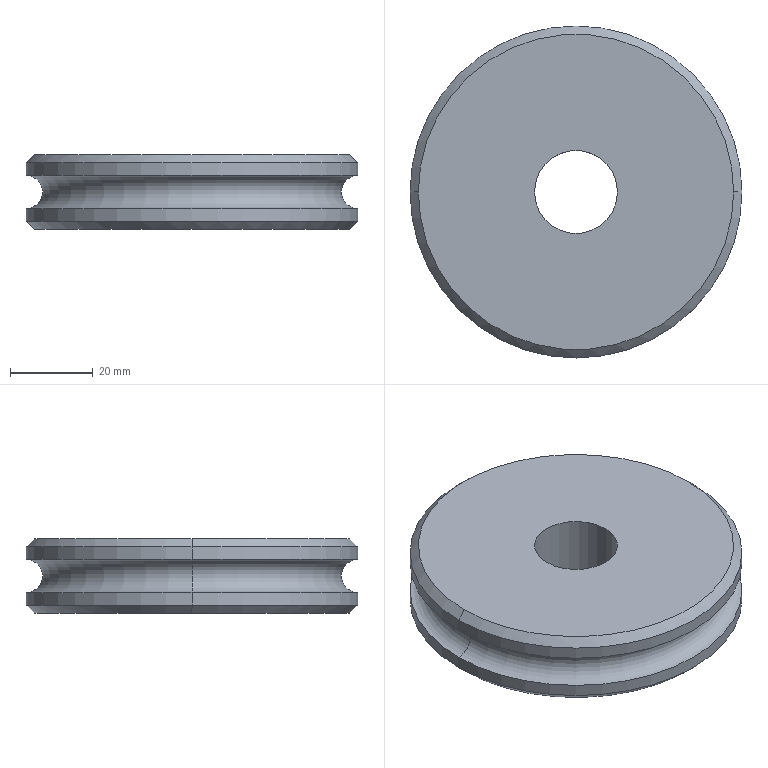Part | Creo | features DATUM PLANE 3, CHAMFER 1, COORDINATE SYSTEM 1, CURVE 1, CUT 1, PROTRUSION 1 | 1 solid | 14 faces | box 80 x 80 x 18 mm | volume 77786 mm3 | cylinder 6 | cone 4 | plane 2 | torus 2 | commonest cylinder face diameters 80 x4 20 x2
STEP:
#1=CARTESIAN_POINT('',(0.,0.,0.));
#2=DIRECTION('',(0.,0.,1.));
#3=DIRECTION('',(1.,0.,0.));
#4=AXIS2_PLACEMENT_3D('',#1,#2,#3);
#5=CARTESIAN_POINT('',(38.,0.,0.));
#6=VERTEX_POINT('',#5);
#7=CARTESIAN_POINT('',(-38.,0.,0.));
#8=VERTEX_POINT('',#7);
#9=CARTESIAN_POINT('',(0.,0.,0.));
#10=DIRECTION('',(0.,0.,-1.));
#11=DIRECTION('',(1.,0.,0.));
#12=AXIS2_PLACEMENT_3D('',#9,#10,#11);
#13=CIRCLE('',#12,38.);
#14=EDGE_CURVE('',#6,#8,#13,.T.);
#15=ORIENTED_EDGE('',*,*,#14,.F.);
#16=CARTESIAN_POINT('',(0.,0.,0.));
#17=DIRECTION('',(0.,0.,-1.));
#18=DIRECTION('',(-1.,0.,0.));
#19=AXIS2_PLACEMENT_3D('',#16,#17,#18);
#20=CIRCLE('',#19,38.);
#21=EDGE_CURVE('',#8,#6,#20,.T.);
#22=ORIENTED_EDGE('',*,*,#21,.F.);
#23=EDGE_LOOP('',(#15,#22));
#24=FACE_OUTER_BOUND('',#23,.F.);
#25=CARTESIAN_POINT('',(10.,0.,0.));
#26=VERTEX_POINT('',#25);
#27=CARTESIAN_POINT('',(-10.,0.,0.));
#28=VERTEX_POINT('',#27);
#29=CARTESIAN_POINT('',(0.,0.,0.));
#30=DIRECTION('',(0.,0.,-1.));
#31=DIRECTION('',(1.,0.,0.));
#32=AXIS2_PLACEMENT_3D('',#29,#30,#31);
#33=CIRCLE('',#32,10.);
#34=EDGE_CURVE('',#26,#28,#33,.T.);
#35=ORIENTED_EDGE('',*,*,#34,.T.);
#36=CARTESIAN_POINT('',(0.,0.,0.));
#37=DIRECTION('',(0.,0.,-1.));
#38=DIRECTION('',(-1.,0.,0.));
#39=AXIS2_PLACEMENT_3D('',#36,#37,#38);
#40=CIRCLE('',#39,10.);
#41=EDGE_CURVE('',#28,#26,#40,.T.);
#42=ORIENTED_EDGE('',*,*,#41,.T.);
#43=EDGE_LOOP('',(#35,#42));
#44=FACE_BOUND('',#43,.F.);
#45=CARTESIAN_POINT('',(0.,0.,0.));
#46=DIRECTION('',(0.,0.,1.));
#47=DIRECTION('',(1.,0.,0.));
#48=AXIS2_PLACEMENT_3D('',#45,#46,#47);
#49=PLANE('',#48);
#50=ADVANCED_FACE('',(#24,#44),#49,.F.);
#51=ORIENTED_EDGE('',*,*,#34,.F.);
#52=CARTESIAN_POINT('',(10.,0.,18.));
#53=VERTEX_POINT('',#52);
#54=CARTESIAN_POINT('',(10.,0.,0.));
#55=DIRECTION('',(0.,0.,1.));
#56=VECTOR('',#55,18.);
#57=LINE('',#54,#56);
#58=EDGE_CURVE('',#26,#53,#57,.T.);
#59=ORIENTED_EDGE('',*,*,#58,.T.);
#60=CARTESIAN_POINT('',(-10.,0.,18.));
#61=VERTEX_POINT('',#60);
#62=CARTESIAN_POINT('',(0.,0.,18.));
#63=DIRECTION('',(0.,0.,-1.));
#64=DIRECTION('',(1.,0.,0.));
#65=AXIS2_PLACEMENT_3D('',#62,#63,#64);
#66=CIRCLE('',#65,10.);
#67=EDGE_CURVE('',#53,#61,#66,.T.);
#68=ORIENTED_EDGE('',*,*,#67,.T.);
#69=CARTESIAN_POINT('',(-10.,0.,0.));
#70=DIRECTION('',(0.,0.,1.));
#71=VECTOR('',#70,18.);
#72=LINE('',#69,#71);
#73=EDGE_CURVE('',#28,#61,#72,.T.);
#74=ORIENTED_EDGE('',*,*,#73,.F.);
#75=EDGE_LOOP('',(#51,#59,#68,#74));
#76=FACE_OUTER_BOUND('',#75,.F.);
#77=CARTESIAN_POINT('',(0.,0.,0.));
#78=DIRECTION('',(0.,0.,1.));
#79=DIRECTION('',(1.,0.,0.));
#80=AXIS2_PLACEMENT_3D('',#77,#78,#79);
#81=CYLINDRICAL_SURFACE('',#80,10.);
#82=ADVANCED_FACE('',(#76),#81,.F.);
#83=ORIENTED_EDGE('',*,*,#41,.F.);
#84=ORIENTED_EDGE('',*,*,#73,.T.);
#85=CARTESIAN_POINT('',(0.,0.,18.));
#86=DIRECTION('',(0.,0.,-1.));
#87=DIRECTION('',(-1.,0.,0.));
#88=AXIS2_PLACEMENT_3D('',#85,#86,#87);
#89=CIRCLE('',#88,10.);
#90=EDGE_CURVE('',#61,#53,#89,.T.);
#91=ORIENTED_EDGE('',*,*,#90,.T.);
#92=ORIENTED_EDGE('',*,*,#58,.F.);
#93=EDGE_LOOP('',(#83,#84,#91,#92));
#94=FACE_OUTER_BOUND('',#93,.F.);
#95=CARTESIAN_POINT('',(0.,0.,0.));
#96=DIRECTION('',(0.,0.,1.));
#97=DIRECTION('',(1.,0.,0.));
#98=AXIS2_PLACEMENT_3D('',#95,#96,#97);
#99=CYLINDRICAL_SURFACE('',#98,10.);
#100=ADVANCED_FACE('',(#94),#99,.F.);
#101=CARTESIAN_POINT('',(-38.,0.,18.));
#102=VERTEX_POINT('',#101);
#103=CARTESIAN_POINT('',(38.,0.,18.));
#104=VERTEX_POINT('',#103);
#105=CARTESIAN_POINT('',(0.,0.,18.));
#106=DIRECTION('',(0.,0.,1.));
#107=DIRECTION('',(-1.,0.,0.));
#108=AXIS2_PLACEMENT_3D('',#105,#106,#107);
#109=CIRCLE('',#108,38.);
#110=EDGE_CURVE('',#102,#104,#109,.T.);
#111=ORIENTED_EDGE('',*,*,#110,.F.);
#112=CARTESIAN_POINT('',(0.,0.,18.));
#113=DIRECTION('',(0.,0.,1.));
#114=DIRECTION('',(1.,0.,0.));
#115=AXIS2_PLACEMENT_3D('',#112,#113,#114);
#116=CIRCLE('',#115,38.);
#117=EDGE_CURVE('',#104,#102,#116,.T.);
#118=ORIENTED_EDGE('',*,*,#117,.F.);
#119=EDGE_LOOP('',(#111,#118));
#120=FACE_OUTER_BOUND('',#119,.F.);
#121=ORIENTED_EDGE('',*,*,#67,.F.);
#122=ORIENTED_EDGE('',*,*,#90,.F.);
#123=EDGE_LOOP('',(#121,#122));
#124=FACE_BOUND('',#123,.F.);
#125=CARTESIAN_POINT('',(0.,0.,18.));
#126=DIRECTION('',(0.,0.,1.));
#127=DIRECTION('',(1.,0.,0.));
#128=AXIS2_PLACEMENT_3D('',#125,#126,#127);
#129=PLANE('',#128);
#130=ADVANCED_FACE('',(#120,#124),#129,.T.);
#131=ORIENTED_EDGE('',*,*,#110,.T.);
#132=CARTESIAN_POINT('',(40.,0.,16.));
#133=VERTEX_POINT('',#132);
#134=CARTESIAN_POINT('',(38.,0.000000005,18.));
#135=DIRECTION('',(0.7071,0.,-0.7071));
#136=VECTOR('',#135,2.828);
#137=LINE('',#134,#136);
#138=EDGE_CURVE('',#104,#133,#137,.T.);
#139=ORIENTED_EDGE('',*,*,#138,.T.);
#140=CARTESIAN_POINT('',(-40.,0.,16.));
#141=VERTEX_POINT('',#140);
#142=CARTESIAN_POINT('',(0.,0.,16.));
#143=DIRECTION('',(0.,0.,1.));
#144=DIRECTION('',(-1.,0.,0.));
#145=AXIS2_PLACEMENT_3D('',#142,#143,#144);
#146=CIRCLE('',#145,40.);
#147=EDGE_CURVE('',#141,#133,#146,.T.);
#148=ORIENTED_EDGE('',*,*,#147,.F.);
#149=CARTESIAN_POINT('',(-38.,-0.000000005,18.));
#150=DIRECTION('',(-0.7071,0.,-0.7071));
#151=VECTOR('',#150,2.828);
#152=LINE('',#149,#151);
#153=EDGE_CURVE('',#102,#141,#152,.T.);
#154=ORIENTED_EDGE('',*,*,#153,.F.);
#155=EDGE_LOOP('',(#131,#139,#148,#154));
#156=FACE_OUTER_BOUND('',#155,.F.);
#157=CARTESIAN_POINT('',(0.,0.,17.));
#158=DIRECTION('',(0.,0.,-1.));
#159=DIRECTION('',(0.,-1.,0.));
#160=AXIS2_PLACEMENT_3D('',#157,#158,#159);
#161=CONICAL_SURFACE('',#160,39.,45.);
#162=ADVANCED_FACE('',(#156),#161,.T.);
#163=ORIENTED_EDGE('',*,*,#117,.T.);
#164=ORIENTED_EDGE('',*,*,#153,.T.);
#165=CARTESIAN_POINT('',(0.,0.,16.));
#166=DIRECTION('',(0.,0.,1.));
#167=DIRECTION('',(1.,0.,0.));
#168=AXIS2_PLACEMENT_3D('',#165,#166,#167);
#169=CIRCLE('',#168,40.);
#170=EDGE_CURVE('',#133,#141,#169,.T.);
#171=ORIENTED_EDGE('',*,*,#170,.F.);
#172=ORIENTED_EDGE('',*,*,#138,.F.);
#173=EDGE_LOOP('',(#163,#164,#171,#172));
#174=FACE_OUTER_BOUND('',#173,.F.);
#175=CARTESIAN_POINT('',(0.,0.,17.));
#176=DIRECTION('',(0.,0.,-1.));
#177=DIRECTION('',(0.,-1.,0.));
#178=AXIS2_PLACEMENT_3D('',#175,#176,#177);
#179=CONICAL_SURFACE('',#178,39.,45.);
#180=ADVANCED_FACE('',(#174),#179,.T.);
#181=ORIENTED_EDGE('',*,*,#170,.T.);
#182=CARTESIAN_POINT('',(-40.,0.,13.));
#183=VERTEX_POINT('',#182);
#184=CARTESIAN_POINT('',(-40.,0.,13.));
#185=DIRECTION('',(0.,-0.000000001,1.));
#186=VECTOR('',#185,3.);
#187=LINE('',#184,#186);
#188=EDGE_CURVE('',#183,#141,#187,.T.);
#189=ORIENTED_EDGE('',*,*,#188,.F.);
#190=CARTESIAN_POINT('',(40.,0.,13.));
#191=VERTEX_POINT('',#190);
#192=CARTESIAN_POINT('',(0.,0.,13.));
#193=DIRECTION('',(0.,0.,1.));
#194=DIRECTION('',(1.,0.,0.));
#195=AXIS2_PLACEMENT_3D('',#192,#193,#194);
#196=CIRCLE('',#195,40.);
#197=EDGE_CURVE('',#191,#183,#196,.T.);
#198=ORIENTED_EDGE('',*,*,#197,.F.);
#199=CARTESIAN_POINT('',(40.,0.,13.));
#200=DIRECTION('',(0.,0.000000001,1.));
#201=VECTOR('',#200,3.);
#202=LINE('',#199,#201);
#203=EDGE_CURVE('',#191,#133,#202,.T.);
#204=ORIENTED_EDGE('',*,*,#203,.T.);
#205=EDGE_LOOP('',(#181,#189,#198,#204));
#206=FACE_OUTER_BOUND('',#205,.F.);
#207=CARTESIAN_POINT('',(0.,0.,0.));
#208=DIRECTION('',(0.,0.,1.));
#209=DIRECTION('',(1.,0.,0.));
#210=AXIS2_PLACEMENT_3D('',#207,#208,#209);
#211=CYLINDRICAL_SURFACE('',#210,40.);
#212=ADVANCED_FACE('',(#206),#211,.T.);
#213=CARTESIAN_POINT('',(-40.,0.,2.));
#214=VERTEX_POINT('',#213);
#215=CARTESIAN_POINT('',(40.,0.,2.));
#216=VERTEX_POINT('',#215);
#217=CARTESIAN_POINT('',(0.,0.,2.));
#218=DIRECTION('',(0.,0.,-1.));
#219=DIRECTION('',(-1.,0.,0.));
#220=AXIS2_PLACEMENT_3D('',#217,#218,#219);
#221=CIRCLE('',#220,40.);
#222=EDGE_CURVE('',#214,#216,#221,.T.);
#223=ORIENTED_EDGE('',*,*,#222,.T.);
#224=CARTESIAN_POINT('',(40.,0.,5.));
#225=VERTEX_POINT('',#224);
#226=CARTESIAN_POINT('',(40.,0.000000004,2.));
#227=DIRECTION('',(0.,-0.000000001,1.));
#228=VECTOR('',#227,3.);
#229=LINE('',#226,#228);
#230=EDGE_CURVE('',#216,#225,#229,.T.);
#231=ORIENTED_EDGE('',*,*,#230,.T.);
#232=CARTESIAN_POINT('',(-40.,0.,5.));
#233=VERTEX_POINT('',#232);
#234=CARTESIAN_POINT('',(0.,0.,5.));
#235=DIRECTION('',(0.,0.,1.));
#236=DIRECTION('',(1.,0.,0.));
#237=AXIS2_PLACEMENT_3D('',#234,#235,#236);
#238=CIRCLE('',#237,40.);
#239=EDGE_CURVE('',#225,#233,#238,.T.);
#240=ORIENTED_EDGE('',*,*,#239,.T.);
#241=CARTESIAN_POINT('',(-40.,-0.000000004,2.));
#242=DIRECTION('',(0.,0.000000001,1.));
#243=VECTOR('',#242,3.);
#244=LINE('',#241,#243);
#245=EDGE_CURVE('',#214,#233,#244,.T.);
#246=ORIENTED_EDGE('',*,*,#245,.F.);
#247=EDGE_LOOP('',(#223,#231,#240,#246));
#248=FACE_OUTER_BOUND('',#247,.F.);
#249=CARTESIAN_POINT('',(0.,0.,0.));
#250=DIRECTION('',(0.,0.,1.));
#251=DIRECTION('',(1.,0.,0.));
#252=AXIS2_PLACEMENT_3D('',#249,#250,#251);
#253=CYLINDRICAL_SURFACE('',#252,40.);
#254=ADVANCED_FACE('',(#248),#253,.T.);
#255=ORIENTED_EDGE('',*,*,#147,.T.);
#256=ORIENTED_EDGE('',*,*,#203,.F.);
#257=CARTESIAN_POINT('',(0.,0.,13.));
#258=DIRECTION('',(0.,0.,1.));
#259=DIRECTION('',(-1.,0.,0.));
#260=AXIS2_PLACEMENT_3D('',#257,#258,#259);
#261=CIRCLE('',#260,40.);
#262=EDGE_CURVE('',#183,#191,#261,.T.);
#263=ORIENTED_EDGE('',*,*,#262,.F.);
#264=ORIENTED_EDGE('',*,*,#188,.T.);
#265=EDGE_LOOP('',(#255,#256,#263,#264));
#266=FACE_OUTER_BOUND('',#265,.F.);
#267=CARTESIAN_POINT('',(0.,0.,0.));
#268=DIRECTION('',(0.,0.,1.));
#269=DIRECTION('',(1.,0.,0.));
#270=AXIS2_PLACEMENT_3D('',#267,#268,#269);
#271=CYLINDRICAL_SURFACE('',#270,40.);
#272=ADVANCED_FACE('',(#266),#271,.T.);
#273=CARTESIAN_POINT('',(0.,0.,2.));
#274=DIRECTION('',(0.,0.,-1.));
#275=DIRECTION('',(1.,0.,0.));
#276=AXIS2_PLACEMENT_3D('',#273,#274,#275);
#277=CIRCLE('',#276,40.);
#278=EDGE_CURVE('',#216,#214,#277,.T.);
#279=ORIENTED_EDGE('',*,*,#278,.T.);
#280=ORIENTED_EDGE('',*,*,#245,.T.);
#281=CARTESIAN_POINT('',(0.,0.,5.));
#282=DIRECTION('',(0.,0.,1.));
#283=DIRECTION('',(-1.,0.,0.));
#284=AXIS2_PLACEMENT_3D('',#281,#282,#283);
#285=CIRCLE('',#284,40.);
#286=EDGE_CURVE('',#233,#225,#285,.T.);
#287=ORIENTED_EDGE('',*,*,#286,.T.);
#288=ORIENTED_EDGE('',*,*,#230,.F.);
#289=EDGE_LOOP('',(#279,#280,#287,#288));
#290=FACE_OUTER_BOUND('',#289,.F.);
#291=CARTESIAN_POINT('',(0.,0.,0.));
#292=DIRECTION('',(0.,0.,1.));
#293=DIRECTION('',(1.,0.,0.));
#294=AXIS2_PLACEMENT_3D('',#291,#292,#293);
#295=CYLINDRICAL_SURFACE('',#294,40.);
#296=ADVANCED_FACE('',(#290),#295,.T.);
#297=ORIENTED_EDGE('',*,*,#262,.T.);
#298=CARTESIAN_POINT('',(40.,0.,9.));
#299=DIRECTION('',(0.,1.,0.));
#300=DIRECTION('',(0.,0.,-1.));
#301=AXIS2_PLACEMENT_3D('',#298,#299,#300);
#302=CIRCLE('',#301,4.);
#303=EDGE_CURVE('',#225,#191,#302,.T.);
#304=ORIENTED_EDGE('',*,*,#303,.F.);
#305=ORIENTED_EDGE('',*,*,#286,.F.);
#306=CARTESIAN_POINT('',(-40.,0.,9.));
#307=DIRECTION('',(0.,-1.,0.));
#308=DIRECTION('',(0.,0.,-1.));
#309=AXIS2_PLACEMENT_3D('',#306,#307,#308);
#310=CIRCLE('',#309,4.);
#311=EDGE_CURVE('',#233,#183,#310,.T.);
#312=ORIENTED_EDGE('',*,*,#311,.T.);
#313=EDGE_LOOP('',(#297,#304,#305,#312));
#314=FACE_OUTER_BOUND('',#313,.F.);
#315=CARTESIAN_POINT('',(0.,0.,9.));
#316=DIRECTION('',(0.,0.,1.));
#317=DIRECTION('',(1.,0.,0.));
#318=AXIS2_PLACEMENT_3D('',#315,#316,#317);
#319=TOROIDAL_SURFACE('',#318,40.,4.);
#320=ADVANCED_FACE('',(#314),#319,.F.);
#321=ORIENTED_EDGE('',*,*,#197,.T.);
#322=ORIENTED_EDGE('',*,*,#311,.F.);
#323=ORIENTED_EDGE('',*,*,#239,.F.);
#324=ORIENTED_EDGE('',*,*,#303,.T.);
#325=EDGE_LOOP('',(#321,#322,#323,#324));
#326=FACE_OUTER_BOUND('',#325,.F.);
#327=CARTESIAN_POINT('',(0.,0.,9.));
#328=DIRECTION('',(0.,0.,1.));
#329=DIRECTION('',(-1.,0.,0.));
#330=AXIS2_PLACEMENT_3D('',#327,#328,#329);
#331=TOROIDAL_SURFACE('',#330,40.,4.);
#332=ADVANCED_FACE('',(#326),#331,.F.);
#333=ORIENTED_EDGE('',*,*,#14,.T.);
#334=CARTESIAN_POINT('',(-38.,-0.000000005,0.));
#335=DIRECTION('',(-0.7071,0.,0.7071));
#336=VECTOR('',#335,2.828);
#337=LINE('',#334,#336);
#338=EDGE_CURVE('',#8,#214,#337,.T.);
#339=ORIENTED_EDGE('',*,*,#338,.T.);
#340=ORIENTED_EDGE('',*,*,#278,.F.);
#341=CARTESIAN_POINT('',(38.,0.000000005,0.));
#342=DIRECTION('',(0.7071,0.,0.7071));
#343=VECTOR('',#342,2.828);
#344=LINE('',#341,#343);
#345=EDGE_CURVE('',#6,#216,#344,.T.);
#346=ORIENTED_EDGE('',*,*,#345,.F.);
#347=EDGE_LOOP('',(#333,#339,#340,#346));
#348=FACE_OUTER_BOUND('',#347,.F.);
#349=CARTESIAN_POINT('',(0.,0.,1.));
#350=DIRECTION('',(0.,0.,1.));
#351=DIRECTION('',(0.,-1.,0.));
#352=AXIS2_PLACEMENT_3D('',#349,#350,#351);
#353=CONICAL_SURFACE('',#352,39.,45.);
#354=ADVANCED_FACE('',(#348),#353,.T.);
#355=ORIENTED_EDGE('',*,*,#21,.T.);
#356=ORIENTED_EDGE('',*,*,#345,.T.);
#357=ORIENTED_EDGE('',*,*,#222,.F.);
#358=ORIENTED_EDGE('',*,*,#338,.F.);
#359=EDGE_LOOP('',(#355,#356,#357,#358));
#360=FACE_OUTER_BOUND('',#359,.F.);
#361=CARTESIAN_POINT('',(0.,0.,1.));
#362=DIRECTION('',(0.,0.,1.));
#363=DIRECTION('',(0.,-1.,0.));
#364=AXIS2_PLACEMENT_3D('',#361,#362,#363);
#365=CONICAL_SURFACE('',#364,39.,45.);
#366=ADVANCED_FACE('',(#360),#365,.T.);
#367=CLOSED_SHELL('',(#50,#82,#100,#130,#162,#180,#212,#254,#272,#296,#320,#332,#354,#366));
#368=MANIFOLD_SOLID_BREP('',#367);
#369=(LENGTH_UNIT()NAMED_UNIT(*)SI_UNIT(.MILLI.,.METRE.));
#370=UNCERTAINTY_MEASURE_WITH_UNIT(LENGTH_MEASURE(0.01146),#369,'','');
#371=(NAMED_UNIT(*)PLANE_ANGLE_UNIT()SI_UNIT($,.RADIAN.));
#372=PLANE_ANGLE_MEASURE_WITH_UNIT(PLANE_ANGLE_MEASURE(0.01745),#371);
#373=(CONVERSION_BASED_UNIT('DEGREE',#372)NAMED_UNIT(*)PLANE_ANGLE_UNIT());
#374=(NAMED_UNIT(*)SI_UNIT($,.STERADIAN.)SOLID_ANGLE_UNIT());
#375=(GEOMETRIC_REPRESENTATION_CONTEXT(3)GLOBAL_UNCERTAINTY_ASSIGNED_CONTEXT((#370))GLOBAL_UNIT_ASSIGNED_CONTEXT((#369,#373,#374))REPRESENTATION_CONTEXT('',''));
#376=ADVANCED_BREP_SHAPE_REPRESENTATION('',(#4,#368),#375);